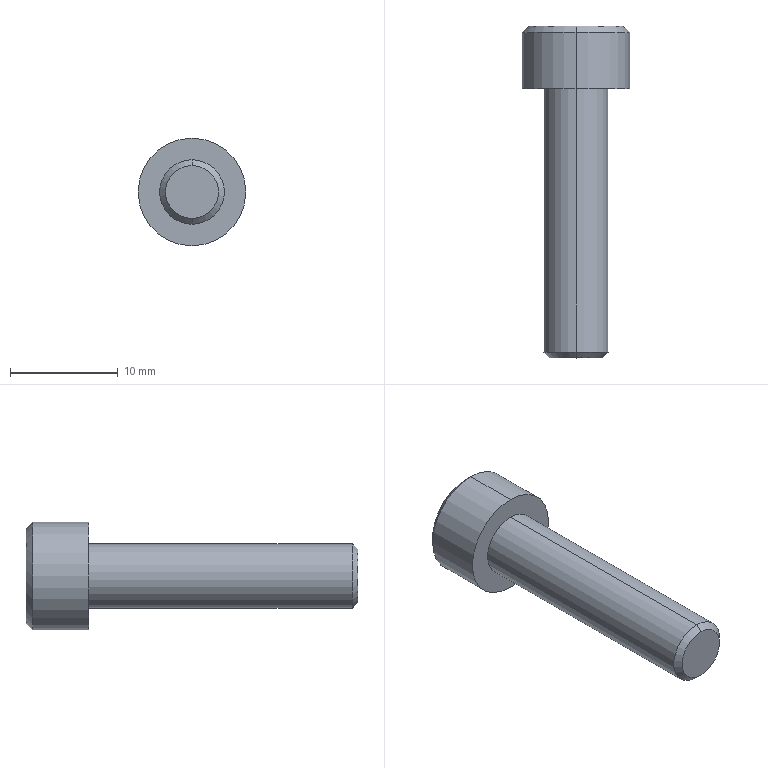Part | STEP file | 0229_Z_MFJC55-20-22_3 | 1 solid | 25 faces | box 10 x 30.82 x 10 mm | volume 1082 mm3 | plane 15 | cone 6 | cylinder 4 | commonest cylinder face diameters 6 x2 10 x2